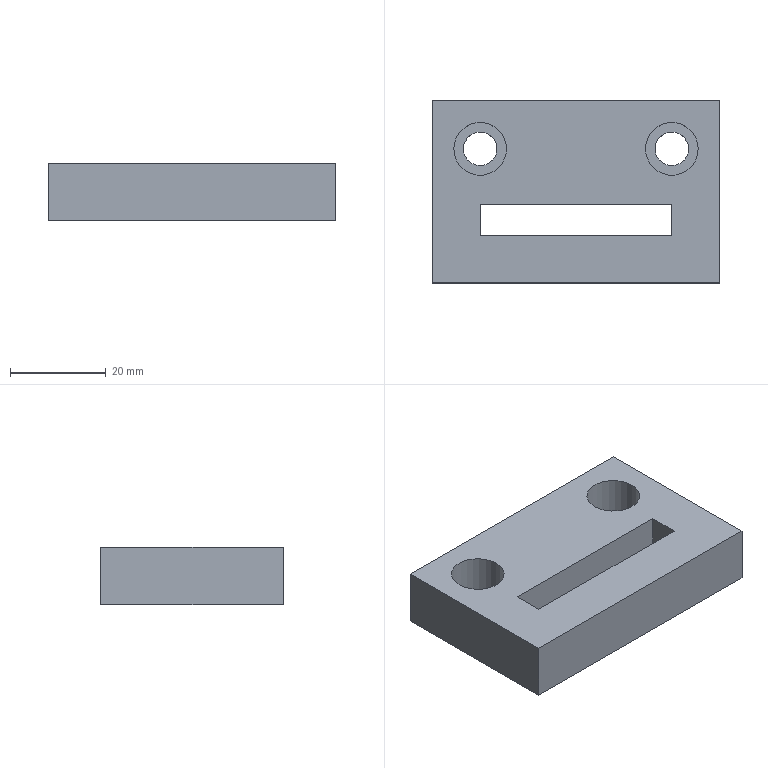Part | STEP file | lll_id702_x_t | 1 solid | 16 faces | box 60 x 38 x 12 mm | volume 22481 mm3 | plane 12 | cylinder 4 | commonest cylinder face diameters 7.009 x2 11.008 x2
STEP:
#1=CARTESIAN_POINT('',(359.5,168.675,-12.));
#2=VERTEX_POINT('',#1);
#3=CARTESIAN_POINT('',(359.5,162.325,-12.));
#4=VERTEX_POINT('',#3);
#5=CARTESIAN_POINT('',(359.5,168.675,-12.));
#6=DIRECTION('',(0.,-1.,0.));
#7=VECTOR('',#6,1.);
#8=LINE('',#5,#7);
#9=EDGE_CURVE('',#2,#4,#8,.T.);
#10=ORIENTED_EDGE('',*,*,#9,.F.);
#11=CARTESIAN_POINT('',(319.5,168.675,-12.));
#12=VERTEX_POINT('',#11);
#13=CARTESIAN_POINT('',(339.5,168.675,-12.));
#14=DIRECTION('',(-1.,0.,0.));
#15=VECTOR('',#14,1.);
#16=LINE('',#13,#15);
#17=EDGE_CURVE('',#2,#12,#16,.T.);
#18=ORIENTED_EDGE('',*,*,#17,.T.);
#19=CARTESIAN_POINT('',(319.5,162.325,-12.));
#20=VERTEX_POINT('',#19);
#21=CARTESIAN_POINT('',(319.5,168.675,-12.));
#22=DIRECTION('',(0.,-1.,0.));
#23=VECTOR('',#22,1.);
#24=LINE('',#21,#23);
#25=EDGE_CURVE('',#12,#20,#24,.T.);
#26=ORIENTED_EDGE('',*,*,#25,.T.);
#27=CARTESIAN_POINT('',(339.5,162.325,-12.));
#28=DIRECTION('',(-1.,0.,0.));
#29=VECTOR('',#28,1.);
#30=LINE('',#27,#29);
#31=EDGE_CURVE('',#4,#20,#30,.T.);
#32=ORIENTED_EDGE('',*,*,#31,.F.);
#33=EDGE_LOOP('',(#10,#18,#26,#32));
#34=FACE_BOUND('',#33,.T.);
#35=CARTESIAN_POINT('',(369.505,190.325,-12.));
#36=VERTEX_POINT('',#35);
#37=CARTESIAN_POINT('',(369.505,152.325,-12.));
#38=VERTEX_POINT('',#37);
#39=CARTESIAN_POINT('',(369.505,165.5,-12.));
#40=DIRECTION('',(0.,-1.,0.));
#41=VECTOR('',#40,1.);
#42=LINE('',#39,#41);
#43=EDGE_CURVE('',#36,#38,#42,.T.);
#44=ORIENTED_EDGE('',*,*,#43,.T.);
#45=CARTESIAN_POINT('',(309.505,152.325,-12.));
#46=VERTEX_POINT('',#45);
#47=CARTESIAN_POINT('',(44.,152.325,-12.));
#48=DIRECTION('',(-1.,0.,0.));
#49=VECTOR('',#48,1.);
#50=LINE('',#47,#49);
#51=EDGE_CURVE('',#38,#46,#50,.T.);
#52=ORIENTED_EDGE('',*,*,#51,.T.);
#53=CARTESIAN_POINT('',(309.505,190.325,-12.));
#54=VERTEX_POINT('',#53);
#55=CARTESIAN_POINT('',(309.505,165.5,-12.));
#56=DIRECTION('',(0.,1.,0.));
#57=VECTOR('',#56,1.);
#58=LINE('',#55,#57);
#59=EDGE_CURVE('',#46,#54,#58,.T.);
#60=ORIENTED_EDGE('',*,*,#59,.T.);
#61=CARTESIAN_POINT('',(44.,190.325,-12.));
#62=DIRECTION('',(1.,0.,0.));
#63=VECTOR('',#62,1.);
#64=LINE('',#61,#63);
#65=EDGE_CURVE('',#54,#36,#64,.T.);
#66=ORIENTED_EDGE('',*,*,#65,.T.);
#67=EDGE_LOOP('',(#44,#52,#60,#66));
#68=FACE_BOUND('',#67,.T.);
#69=CARTESIAN_POINT('',(323.009,180.325,-12.));
#70=VERTEX_POINT('',#69);
#71=CARTESIAN_POINT('',(319.505,180.325,-12.));
#72=DIRECTION('',(0.,0.,1.));
#73=DIRECTION('',(1.,0.,0.));
#74=AXIS2_PLACEMENT_3D('',#71,#72,#73);
#75=CIRCLE('',#74,3.505);
#76=EDGE_CURVE('',#70,#70,#75,.T.);
#77=ORIENTED_EDGE('',*,*,#76,.T.);
#78=EDGE_LOOP('',(#77));
#79=FACE_BOUND('',#78,.T.);
#80=CARTESIAN_POINT('',(356.,180.325,-12.));
#81=VERTEX_POINT('',#80);
#82=CARTESIAN_POINT('',(359.505,180.325,-12.));
#83=DIRECTION('',(0.,0.,-1.));
#84=DIRECTION('',(-1.,0.,0.));
#85=AXIS2_PLACEMENT_3D('',#82,#83,#84);
#86=CIRCLE('',#85,3.505);
#87=EDGE_CURVE('',#81,#81,#86,.T.);
#88=ORIENTED_EDGE('',*,*,#87,.F.);
#89=EDGE_LOOP('',(#88));
#90=FACE_BOUND('',#89,.T.);
#91=CARTESIAN_POINT('',(329.505,165.5,-12.));
#92=DIRECTION('',(0.,0.,-1.));
#93=DIRECTION('',(1.,0.,0.));
#94=AXIS2_PLACEMENT_3D('',#91,#92,#93);
#95=PLANE('',#94);
#96=ADVANCED_FACE('',(#34,#68,#79,#90),#95,.T.);
#97=CARTESIAN_POINT('',(369.505,190.325,0.));
#98=VERTEX_POINT('',#97);
#99=CARTESIAN_POINT('',(309.505,190.325,0.));
#100=VERTEX_POINT('',#99);
#101=CARTESIAN_POINT('',(44.,190.325,0.));
#102=DIRECTION('',(-1.,0.,0.));
#103=VECTOR('',#102,1.);
#104=LINE('',#101,#103);
#105=EDGE_CURVE('',#98,#100,#104,.T.);
#106=ORIENTED_EDGE('',*,*,#105,.T.);
#107=CARTESIAN_POINT('',(309.505,152.325,0.));
#108=VERTEX_POINT('',#107);
#109=CARTESIAN_POINT('',(309.505,165.5,0.));
#110=DIRECTION('',(0.,-1.,0.));
#111=VECTOR('',#110,1.);
#112=LINE('',#109,#111);
#113=EDGE_CURVE('',#100,#108,#112,.T.);
#114=ORIENTED_EDGE('',*,*,#113,.T.);
#115=CARTESIAN_POINT('',(369.505,152.325,0.));
#116=VERTEX_POINT('',#115);
#117=CARTESIAN_POINT('',(44.,152.325,0.));
#118=DIRECTION('',(1.,0.,0.));
#119=VECTOR('',#118,1.);
#120=LINE('',#117,#119);
#121=EDGE_CURVE('',#108,#116,#120,.T.);
#122=ORIENTED_EDGE('',*,*,#121,.T.);
#123=CARTESIAN_POINT('',(369.505,165.5,0.));
#124=DIRECTION('',(0.,1.,0.));
#125=VECTOR('',#124,1.);
#126=LINE('',#123,#125);
#127=EDGE_CURVE('',#116,#98,#126,.T.);
#128=ORIENTED_EDGE('',*,*,#127,.T.);
#129=EDGE_LOOP('',(#106,#114,#122,#128));
#130=FACE_BOUND('',#129,.T.);
#131=CARTESIAN_POINT('',(359.5,162.325,0.));
#132=VERTEX_POINT('',#131);
#133=CARTESIAN_POINT('',(319.5,162.325,0.));
#134=VERTEX_POINT('',#133);
#135=CARTESIAN_POINT('',(339.5,162.325,0.));
#136=DIRECTION('',(-1.,0.,0.));
#137=VECTOR('',#136,1.);
#138=LINE('',#135,#137);
#139=EDGE_CURVE('',#132,#134,#138,.T.);
#140=ORIENTED_EDGE('',*,*,#139,.T.);
#141=CARTESIAN_POINT('',(319.5,168.675,0.));
#142=VERTEX_POINT('',#141);
#143=CARTESIAN_POINT('',(319.5,168.675,0.));
#144=DIRECTION('',(0.,-1.,0.));
#145=VECTOR('',#144,1.);
#146=LINE('',#143,#145);
#147=EDGE_CURVE('',#142,#134,#146,.T.);
#148=ORIENTED_EDGE('',*,*,#147,.F.);
#149=CARTESIAN_POINT('',(359.5,168.675,0.));
#150=VERTEX_POINT('',#149);
#151=CARTESIAN_POINT('',(339.5,168.675,0.));
#152=DIRECTION('',(-1.,0.,0.));
#153=VECTOR('',#152,1.);
#154=LINE('',#151,#153);
#155=EDGE_CURVE('',#150,#142,#154,.T.);
#156=ORIENTED_EDGE('',*,*,#155,.F.);
#157=CARTESIAN_POINT('',(359.5,168.675,0.));
#158=DIRECTION('',(0.,-1.,0.));
#159=VECTOR('',#158,1.);
#160=LINE('',#157,#159);
#161=EDGE_CURVE('',#150,#132,#160,.T.);
#162=ORIENTED_EDGE('',*,*,#161,.T.);
#163=EDGE_LOOP('',(#140,#148,#156,#162));
#164=FACE_BOUND('',#163,.T.);
#165=CARTESIAN_POINT('',(325.009,180.325,0.));
#166=VERTEX_POINT('',#165);
#167=CARTESIAN_POINT('',(319.505,180.325,0.));
#168=DIRECTION('',(0.,0.,-1.));
#169=DIRECTION('',(1.,0.,0.));
#170=AXIS2_PLACEMENT_3D('',#167,#168,#169);
#171=CIRCLE('',#170,5.504);
#172=EDGE_CURVE('',#166,#166,#171,.T.);
#173=ORIENTED_EDGE('',*,*,#172,.T.);
#174=EDGE_LOOP('',(#173));
#175=FACE_BOUND('',#174,.T.);
#176=CARTESIAN_POINT('',(354.001,180.325,0.));
#177=VERTEX_POINT('',#176);
#178=CARTESIAN_POINT('',(359.505,180.325,0.));
#179=DIRECTION('',(0.,0.,1.));
#180=DIRECTION('',(-1.,0.,0.));
#181=AXIS2_PLACEMENT_3D('',#178,#179,#180);
#182=CIRCLE('',#181,5.504);
#183=EDGE_CURVE('',#177,#177,#182,.T.);
#184=ORIENTED_EDGE('',*,*,#183,.F.);
#185=EDGE_LOOP('',(#184));
#186=FACE_BOUND('',#185,.T.);
#187=CARTESIAN_POINT('',(329.505,165.5,0.));
#188=DIRECTION('',(0.,0.,1.));
#189=DIRECTION('',(-1.,0.,0.));
#190=AXIS2_PLACEMENT_3D('',#187,#188,#189);
#191=PLANE('',#190);
#192=ADVANCED_FACE('',(#130,#164,#175,#186),#191,.T.);
#193=CARTESIAN_POINT('',(369.505,190.325,0.));
#194=DIRECTION('',(0.,0.,1.));
#195=VECTOR('',#194,1.);
#196=LINE('',#193,#195);
#197=EDGE_CURVE('',#36,#98,#196,.T.);
#198=ORIENTED_EDGE('',*,*,#197,.F.);
#199=ORIENTED_EDGE('',*,*,#65,.F.);
#200=CARTESIAN_POINT('',(309.505,190.325,-12.));
#201=DIRECTION('',(0.,0.,1.));
#202=VECTOR('',#201,1.);
#203=LINE('',#200,#202);
#204=EDGE_CURVE('',#54,#100,#203,.T.);
#205=ORIENTED_EDGE('',*,*,#204,.T.);
#206=ORIENTED_EDGE('',*,*,#105,.F.);
#207=EDGE_LOOP('',(#198,#199,#205,#206));
#208=FACE_OUTER_BOUND('',#207,.T.);
#209=CARTESIAN_POINT('',(44.,190.325,0.));
#210=DIRECTION('',(0.,1.,0.));
#211=DIRECTION('',(0.,0.,1.));
#212=AXIS2_PLACEMENT_3D('',#209,#210,#211);
#213=PLANE('',#212);
#214=ADVANCED_FACE('',(#208),#213,.T.);
#215=ORIENTED_EDGE('',*,*,#204,.F.);
#216=ORIENTED_EDGE('',*,*,#59,.F.);
#217=CARTESIAN_POINT('',(309.505,152.325,0.));
#218=DIRECTION('',(0.,0.,1.));
#219=VECTOR('',#218,1.);
#220=LINE('',#217,#219);
#221=EDGE_CURVE('',#46,#108,#220,.T.);
#222=ORIENTED_EDGE('',*,*,#221,.T.);
#223=ORIENTED_EDGE('',*,*,#113,.F.);
#224=EDGE_LOOP('',(#215,#216,#222,#223));
#225=FACE_OUTER_BOUND('',#224,.T.);
#226=CARTESIAN_POINT('',(309.505,165.5,-12.));
#227=DIRECTION('',(-1.,0.,0.));
#228=DIRECTION('',(0.,0.,-1.));
#229=AXIS2_PLACEMENT_3D('',#226,#227,#228);
#230=PLANE('',#229);
#231=ADVANCED_FACE('',(#225),#230,.T.);
#232=ORIENTED_EDGE('',*,*,#221,.F.);
#233=ORIENTED_EDGE('',*,*,#51,.F.);
#234=CARTESIAN_POINT('',(369.505,152.325,-12.));
#235=DIRECTION('',(0.,0.,1.));
#236=VECTOR('',#235,1.);
#237=LINE('',#234,#236);
#238=EDGE_CURVE('',#38,#116,#237,.T.);
#239=ORIENTED_EDGE('',*,*,#238,.T.);
#240=ORIENTED_EDGE('',*,*,#121,.F.);
#241=EDGE_LOOP('',(#232,#233,#239,#240));
#242=FACE_OUTER_BOUND('',#241,.T.);
#243=CARTESIAN_POINT('',(44.,152.325,0.));
#244=DIRECTION('',(0.,1.,0.));
#245=DIRECTION('',(0.,0.,1.));
#246=AXIS2_PLACEMENT_3D('',#243,#244,#245);
#247=PLANE('',#246);
#248=ADVANCED_FACE('',(#242),#247,.F.);
#249=ORIENTED_EDGE('',*,*,#43,.F.);
#250=ORIENTED_EDGE('',*,*,#197,.T.);
#251=ORIENTED_EDGE('',*,*,#127,.F.);
#252=ORIENTED_EDGE('',*,*,#238,.F.);
#253=EDGE_LOOP('',(#249,#250,#251,#252));
#254=FACE_OUTER_BOUND('',#253,.T.);
#255=CARTESIAN_POINT('',(369.505,165.5,-12.));
#256=DIRECTION('',(1.,0.,0.));
#257=DIRECTION('',(0.,0.,1.));
#258=AXIS2_PLACEMENT_3D('',#255,#256,#257);
#259=PLANE('',#258);
#260=ADVANCED_FACE('',(#254),#259,.T.);
#261=CARTESIAN_POINT('',(319.5,162.325,-12.));
#262=DIRECTION('',(0.,0.,-1.));
#263=VECTOR('',#262,1.);
#264=LINE('',#261,#263);
#265=EDGE_CURVE('',#134,#20,#264,.T.);
#266=ORIENTED_EDGE('',*,*,#265,.T.);
#267=ORIENTED_EDGE('',*,*,#25,.F.);
#268=CARTESIAN_POINT('',(319.5,168.675,-12.));
#269=DIRECTION('',(0.,0.,-1.));
#270=VECTOR('',#269,1.);
#271=LINE('',#268,#270);
#272=EDGE_CURVE('',#142,#12,#271,.T.);
#273=ORIENTED_EDGE('',*,*,#272,.F.);
#274=ORIENTED_EDGE('',*,*,#147,.T.);
#275=EDGE_LOOP('',(#266,#267,#273,#274));
#276=FACE_OUTER_BOUND('',#275,.T.);
#277=CARTESIAN_POINT('',(319.5,168.675,-12.));
#278=DIRECTION('',(-1.,0.,0.));
#279=DIRECTION('',(0.,0.,-1.));
#280=AXIS2_PLACEMENT_3D('',#277,#278,#279);
#281=PLANE('',#280);
#282=ADVANCED_FACE('',(#276),#281,.F.);
#283=CARTESIAN_POINT('',(359.5,162.325,-12.));
#284=DIRECTION('',(0.,0.,-1.));
#285=VECTOR('',#284,1.);
#286=LINE('',#283,#285);
#287=EDGE_CURVE('',#132,#4,#286,.T.);
#288=ORIENTED_EDGE('',*,*,#287,.F.);
#289=ORIENTED_EDGE('',*,*,#161,.F.);
#290=CARTESIAN_POINT('',(359.5,168.675,-12.));
#291=DIRECTION('',(0.,0.,-1.));
#292=VECTOR('',#291,1.);
#293=LINE('',#290,#292);
#294=EDGE_CURVE('',#150,#2,#293,.T.);
#295=ORIENTED_EDGE('',*,*,#294,.T.);
#296=ORIENTED_EDGE('',*,*,#9,.T.);
#297=EDGE_LOOP('',(#288,#289,#295,#296));
#298=FACE_OUTER_BOUND('',#297,.T.);
#299=CARTESIAN_POINT('',(359.5,168.675,-12.));
#300=DIRECTION('',(-1.,0.,0.));
#301=DIRECTION('',(0.,0.,-1.));
#302=AXIS2_PLACEMENT_3D('',#299,#300,#301);
#303=PLANE('',#302);
#304=ADVANCED_FACE('',(#298),#303,.T.);
#305=ORIENTED_EDGE('',*,*,#272,.T.);
#306=ORIENTED_EDGE('',*,*,#17,.F.);
#307=ORIENTED_EDGE('',*,*,#294,.F.);
#308=ORIENTED_EDGE('',*,*,#155,.T.);
#309=EDGE_LOOP('',(#305,#306,#307,#308));
#310=FACE_OUTER_BOUND('',#309,.T.);
#311=CARTESIAN_POINT('',(44.,168.675,0.));
#312=DIRECTION('',(0.,1.,0.));
#313=DIRECTION('',(0.,0.,1.));
#314=AXIS2_PLACEMENT_3D('',#311,#312,#313);
#315=PLANE('',#314);
#316=ADVANCED_FACE('',(#310),#315,.F.);
#317=ORIENTED_EDGE('',*,*,#265,.F.);
#318=ORIENTED_EDGE('',*,*,#139,.F.);
#319=ORIENTED_EDGE('',*,*,#287,.T.);
#320=ORIENTED_EDGE('',*,*,#31,.T.);
#321=EDGE_LOOP('',(#317,#318,#319,#320));
#322=FACE_OUTER_BOUND('',#321,.T.);
#323=CARTESIAN_POINT('',(44.,162.325,0.));
#324=DIRECTION('',(0.,1.,0.));
#325=DIRECTION('',(0.,0.,1.));
#326=AXIS2_PLACEMENT_3D('',#323,#324,#325);
#327=PLANE('',#326);
#328=ADVANCED_FACE('',(#322),#327,.T.);
#329=CARTESIAN_POINT('',(323.009,180.325,-8.));
#330=VERTEX_POINT('',#329);
#331=CARTESIAN_POINT('',(319.505,180.325,-8.));
#332=DIRECTION('',(0.,0.,-1.));
#333=DIRECTION('',(1.,0.,0.));
#334=AXIS2_PLACEMENT_3D('',#331,#332,#333);
#335=CIRCLE('',#334,3.505);
#336=EDGE_CURVE('',#330,#330,#335,.T.);
#337=ORIENTED_EDGE('',*,*,#336,.F.);
#338=EDGE_LOOP('',(#337));
#339=FACE_BOUND('',#338,.T.);
#340=ORIENTED_EDGE('',*,*,#76,.F.);
#341=EDGE_LOOP('',(#340));
#342=FACE_BOUND('',#341,.T.);
#343=CARTESIAN_POINT('',(319.505,180.325,0.));
#344=DIRECTION('',(0.,0.,-1.));
#345=DIRECTION('',(-1.,0.,0.));
#346=AXIS2_PLACEMENT_3D('',#343,#344,#345);
#347=CYLINDRICAL_SURFACE('',#346,3.505);
#348=ADVANCED_FACE('',(#339,#342),#347,.F.);
#349=ORIENTED_EDGE('',*,*,#336,.T.);
#350=EDGE_LOOP('',(#349));
#351=FACE_BOUND('',#350,.T.);
#352=CARTESIAN_POINT('',(325.009,180.325,-8.));
#353=VERTEX_POINT('',#352);
#354=CARTESIAN_POINT('',(319.505,180.325,-8.));
#355=DIRECTION('',(0.,0.,-1.));
#356=DIRECTION('',(1.,0.,0.));
#357=AXIS2_PLACEMENT_3D('',#354,#355,#356);
#358=CIRCLE('',#357,5.504);
#359=EDGE_CURVE('',#353,#353,#358,.T.);
#360=ORIENTED_EDGE('',*,*,#359,.F.);
#361=EDGE_LOOP('',(#360));
#362=FACE_BOUND('',#361,.T.);
#363=CARTESIAN_POINT('',(319.505,180.325,-8.));
#364=DIRECTION('',(0.,0.,-1.));
#365=DIRECTION('',(-1.,0.,0.));
#366=AXIS2_PLACEMENT_3D('',#363,#364,#365);
#367=PLANE('',#366);
#368=ADVANCED_FACE('',(#351,#362),#367,.F.);
#369=ORIENTED_EDGE('',*,*,#359,.T.);
#370=EDGE_LOOP('',(#369));
#371=FACE_BOUND('',#370,.T.);
#372=ORIENTED_EDGE('',*,*,#172,.F.);
#373=EDGE_LOOP('',(#372));
#374=FACE_BOUND('',#373,.T.);
#375=CARTESIAN_POINT('',(319.505,180.325,0.));
#376=DIRECTION('',(0.,0.,-1.));
#377=DIRECTION('',(-1.,0.,0.));
#378=AXIS2_PLACEMENT_3D('',#375,#376,#377);
#379=CYLINDRICAL_SURFACE('',#378,5.504);
#380=ADVANCED_FACE('',(#371,#374),#379,.F.);
#381=CARTESIAN_POINT('',(356.,180.325,-8.));
#382=VERTEX_POINT('',#381);
#383=CARTESIAN_POINT('',(359.505,180.325,-8.));
#384=DIRECTION('',(0.,0.,1.));
#385=DIRECTION('',(-1.,0.,0.));
#386=AXIS2_PLACEMENT_3D('',#383,#384,#385);
#387=CIRCLE('',#386,3.505);
#388=EDGE_CURVE('',#382,#382,#387,.T.);
#389=ORIENTED_EDGE('',*,*,#388,.T.);
#390=EDGE_LOOP('',(#389));
#391=FACE_BOUND('',#390,.T.);
#392=ORIENTED_EDGE('',*,*,#87,.T.);
#393=EDGE_LOOP('',(#392));
#394=FACE_BOUND('',#393,.T.);
#395=CARTESIAN_POINT('',(359.505,180.325,0.));
#396=DIRECTION('',(0.,0.,-1.));
#397=DIRECTION('',(1.,0.,0.));
#398=AXIS2_PLACEMENT_3D('',#395,#396,#397);
#399=CYLINDRICAL_SURFACE('',#398,3.505);
#400=ADVANCED_FACE('',(#391,#394),#399,.F.);
#401=ORIENTED_EDGE('',*,*,#388,.F.);
#402=EDGE_LOOP('',(#401));
#403=FACE_BOUND('',#402,.T.);
#404=CARTESIAN_POINT('',(354.001,180.325,-8.));
#405=VERTEX_POINT('',#404);
#406=CARTESIAN_POINT('',(359.505,180.325,-8.));
#407=DIRECTION('',(0.,0.,1.));
#408=DIRECTION('',(-1.,0.,0.));
#409=AXIS2_PLACEMENT_3D('',#406,#407,#408);
#410=CIRCLE('',#409,5.504);
#411=EDGE_CURVE('',#405,#405,#410,.T.);
#412=ORIENTED_EDGE('',*,*,#411,.T.);
#413=EDGE_LOOP('',(#412));
#414=FACE_BOUND('',#413,.T.);
#415=CARTESIAN_POINT('',(359.505,180.325,-8.));
#416=DIRECTION('',(0.,0.,-1.));
#417=DIRECTION('',(1.,0.,0.));
#418=AXIS2_PLACEMENT_3D('',#415,#416,#417);
#419=PLANE('',#418);
#420=ADVANCED_FACE('',(#403,#414),#419,.F.);
#421=ORIENTED_EDGE('',*,*,#411,.F.);
#422=EDGE_LOOP('',(#421));
#423=FACE_BOUND('',#422,.T.);
#424=ORIENTED_EDGE('',*,*,#183,.T.);
#425=EDGE_LOOP('',(#424));
#426=FACE_BOUND('',#425,.T.);
#427=CARTESIAN_POINT('',(359.505,180.325,0.));
#428=DIRECTION('',(0.,0.,-1.));
#429=DIRECTION('',(1.,0.,0.));
#430=AXIS2_PLACEMENT_3D('',#427,#428,#429);
#431=CYLINDRICAL_SURFACE('',#430,5.504);
#432=ADVANCED_FACE('',(#423,#426),#431,.F.);
#433=CLOSED_SHELL('',(#96,#192,#214,#231,#248,#260,#282,#304,#316,#328,#348,#368,#380,#400,#420,#432));
#434=MANIFOLD_SOLID_BREP('',#433);
#435=(LENGTH_UNIT()NAMED_UNIT(*)SI_UNIT(.MILLI.,.METRE.));
#436=UNCERTAINTY_MEASURE_WITH_UNIT(LENGTH_MEASURE(0.00002),#435,'','');
#437=(NAMED_UNIT(*)PLANE_ANGLE_UNIT()SI_UNIT($,.RADIAN.));
#438=PLANE_ANGLE_MEASURE_WITH_UNIT(PLANE_ANGLE_MEASURE(0.01745),#437);
#439=DIMENSIONAL_EXPONENTS(0.,0.,0.,0.,0.,0.,0.);
#440=(CONVERSION_BASED_UNIT('DEGREE',#438)NAMED_UNIT(#439)PLANE_ANGLE_UNIT());
#441=(NAMED_UNIT(*)SI_UNIT($,.STERADIAN.)SOLID_ANGLE_UNIT());
#442=(GEOMETRIC_REPRESENTATION_CONTEXT(3)GLOBAL_UNCERTAINTY_ASSIGNED_CONTEXT((#436))GLOBAL_UNIT_ASSIGNED_CONTEXT((#435,#440,#441))REPRESENTATION_CONTEXT('',''));
#443=ADVANCED_BREP_SHAPE_REPRESENTATION('',(#434),#442);